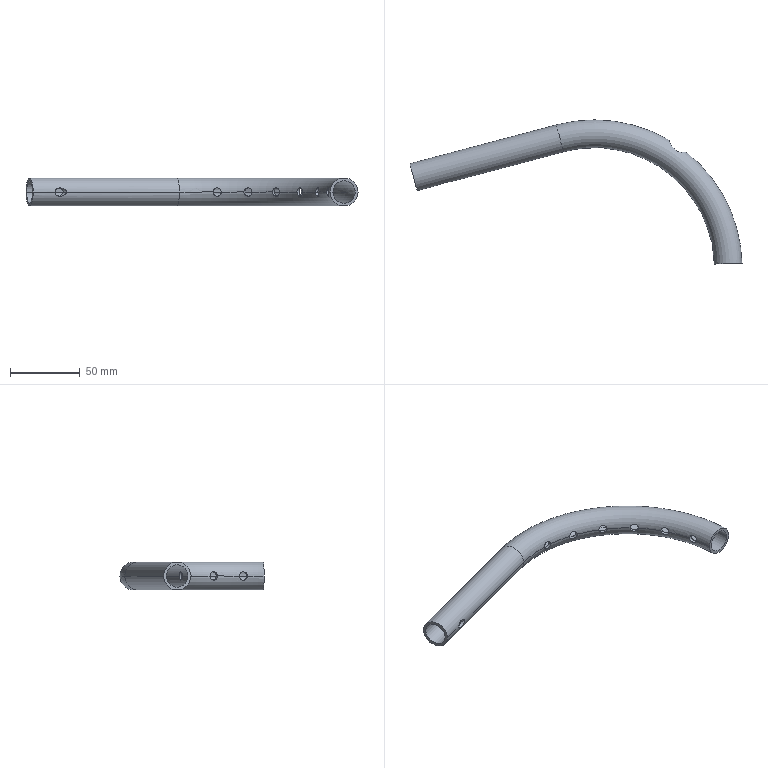Part | SolidWorks | features RevCut 2, CirPattern 1, Cut 1, RefAxis 1, Sweep 1 | 1 solid | 28 faces | box 238.083 x 103.353 x 20 mm | volume 30963 mm3 | cylinder 18 | torus 4 | plane 4 | spline 2 | commonest cylinder face diameters 6 x14 16 x2 20 x2